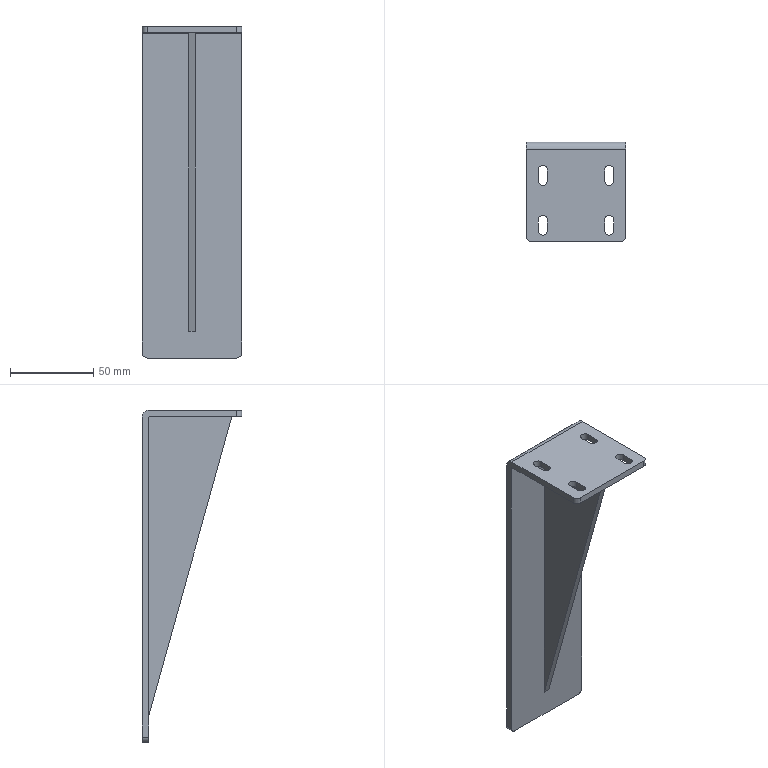Part | STEP file | HJDX-302 | 2 solids | 35 faces | box 60 x 60 x 200 mm | volume 78199 mm3 | plane 21 | cylinder 14 | commonest cylinder face diameters 5.5 x8 6 x4 1 x1 9 x1
STEP:
#1=CARTESIAN_POINT('',(-27.,56.,-200.));
#2=VERTEX_POINT('',#1);
#3=CARTESIAN_POINT('',(-30.,56.,-197.));
#4=VERTEX_POINT('',#3);
#5=CARTESIAN_POINT('',(-27.,56.,-197.));
#6=DIRECTION('',(0.,1.,0.));
#7=DIRECTION('',(0.,0.,1.));
#8=AXIS2_PLACEMENT_3D('',#5,#6,#7);
#9=CIRCLE('',#8,3.);
#10=EDGE_CURVE('',#2,#4,#9,.T.);
#11=ORIENTED_EDGE('',*,*,#10,.F.);
#12=CARTESIAN_POINT('',(27.,56.,-200.));
#13=VERTEX_POINT('',#12);
#14=CARTESIAN_POINT('',(30.,56.,-200.));
#15=DIRECTION('',(-1.,0.,0.));
#16=VECTOR('',#15,1000.);
#17=LINE('',#14,#16);
#18=EDGE_CURVE('',#13,#2,#17,.T.);
#19=ORIENTED_EDGE('',*,*,#18,.F.);
#20=CARTESIAN_POINT('',(30.,56.,-197.));
#21=VERTEX_POINT('',#20);
#22=CARTESIAN_POINT('',(27.,56.,-197.));
#23=DIRECTION('',(0.,1.,0.));
#24=DIRECTION('',(0.,0.,-1.));
#25=AXIS2_PLACEMENT_3D('',#22,#23,#24);
#26=CIRCLE('',#25,3.);
#27=EDGE_CURVE('',#21,#13,#26,.T.);
#28=ORIENTED_EDGE('',*,*,#27,.F.);
#29=CARTESIAN_POINT('',(30.,56.,-4.5));
#30=VERTEX_POINT('',#29);
#31=CARTESIAN_POINT('',(30.,56.,0.));
#32=DIRECTION('',(0.,0.,-1.));
#33=VECTOR('',#32,1000.);
#34=LINE('',#31,#33);
#35=EDGE_CURVE('',#30,#21,#34,.T.);
#36=ORIENTED_EDGE('',*,*,#35,.F.);
#37=CARTESIAN_POINT('',(-30.,56.,-4.5));
#38=VERTEX_POINT('',#37);
#39=CARTESIAN_POINT('',(30.,56.,-4.5));
#40=DIRECTION('',(1.,0.,0.));
#41=VECTOR('',#40,1000.);
#42=LINE('',#39,#41);
#43=EDGE_CURVE('',#38,#30,#42,.T.);
#44=ORIENTED_EDGE('',*,*,#43,.F.);
#45=CARTESIAN_POINT('',(-30.,56.,0.));
#46=DIRECTION('',(0.,0.,1.));
#47=VECTOR('',#46,1000.);
#48=LINE('',#45,#47);
#49=EDGE_CURVE('',#4,#38,#48,.T.);
#50=ORIENTED_EDGE('',*,*,#49,.F.);
#51=EDGE_LOOP('',(#11,#19,#28,#36,#44,#50));
#52=FACE_OUTER_BOUND('',#51,.T.);
#53=CARTESIAN_POINT('',(30.,56.,0.));
#54=DIRECTION('',(0.,1.,0.));
#55=DIRECTION('',(0.,0.,1.));
#56=AXIS2_PLACEMENT_3D('',#53,#54,#55);
#57=PLANE('',#56);
#58=ADVANCED_FACE('',(#52),#57,.F.);
#59=CARTESIAN_POINT('',(-30.,60.,-197.));
#60=VERTEX_POINT('',#59);
#61=CARTESIAN_POINT('',(-30.,55.5,-197.));
#62=DIRECTION('',(0.,1.,0.));
#63=VECTOR('',#62,1000.);
#64=LINE('',#61,#63);
#65=EDGE_CURVE('',#4,#60,#64,.T.);
#66=ORIENTED_EDGE('',*,*,#65,.F.);
#67=ORIENTED_EDGE('',*,*,#49,.T.);
#68=CARTESIAN_POINT('',(-30.,55.5,-4.));
#69=VERTEX_POINT('',#68);
#70=CARTESIAN_POINT('',(-30.,55.5,-4.5));
#71=DIRECTION('',(1.,0.,0.));
#72=DIRECTION('',(0.,0.,1.));
#73=AXIS2_PLACEMENT_3D('',#70,#71,#72);
#74=CIRCLE('',#73,0.5);
#75=EDGE_CURVE('',#38,#69,#74,.T.);
#76=ORIENTED_EDGE('',*,*,#75,.T.);
#77=CARTESIAN_POINT('',(-30.,3.,-4.));
#78=VERTEX_POINT('',#77);
#79=CARTESIAN_POINT('',(-30.,0.,-4.));
#80=DIRECTION('',(0.,-1.,0.));
#81=VECTOR('',#80,1000.);
#82=LINE('',#79,#81);
#83=EDGE_CURVE('',#69,#78,#82,.T.);
#84=ORIENTED_EDGE('',*,*,#83,.T.);
#85=CARTESIAN_POINT('',(-30.,3.,0.));
#86=VERTEX_POINT('',#85);
#87=CARTESIAN_POINT('',(-30.,3.,-4.5));
#88=DIRECTION('',(0.,0.,1.));
#89=VECTOR('',#88,1000.);
#90=LINE('',#87,#89);
#91=EDGE_CURVE('',#78,#86,#90,.T.);
#92=ORIENTED_EDGE('',*,*,#91,.T.);
#93=CARTESIAN_POINT('',(-30.,55.5,0.));
#94=VERTEX_POINT('',#93);
#95=CARTESIAN_POINT('',(-30.,56.,0.));
#96=DIRECTION('',(0.,1.,0.));
#97=VECTOR('',#96,1000.);
#98=LINE('',#95,#97);
#99=EDGE_CURVE('',#86,#94,#98,.T.);
#100=ORIENTED_EDGE('',*,*,#99,.T.);
#101=CARTESIAN_POINT('',(-30.,60.,-4.5));
#102=VERTEX_POINT('',#101);
#103=CARTESIAN_POINT('',(-30.,55.5,-4.5));
#104=DIRECTION('',(-1.,0.,0.));
#105=DIRECTION('',(0.,0.,1.));
#106=AXIS2_PLACEMENT_3D('',#103,#104,#105);
#107=CIRCLE('',#106,4.5);
#108=EDGE_CURVE('',#94,#102,#107,.T.);
#109=ORIENTED_EDGE('',*,*,#108,.T.);
#110=CARTESIAN_POINT('',(-30.,60.,-4.5));
#111=DIRECTION('',(0.,0.,1.));
#112=VECTOR('',#111,1000.);
#113=LINE('',#110,#112);
#114=EDGE_CURVE('',#60,#102,#113,.T.);
#115=ORIENTED_EDGE('',*,*,#114,.F.);
#116=EDGE_LOOP('',(#66,#67,#76,#84,#92,#100,#109,#115));
#117=FACE_OUTER_BOUND('',#116,.T.);
#118=CARTESIAN_POINT('',(-30.,55.5,-4.5));
#119=DIRECTION('',(1.,0.,0.));
#120=DIRECTION('',(0.,0.,-1.));
#121=AXIS2_PLACEMENT_3D('',#118,#119,#120);
#122=PLANE('',#121);
#123=ADVANCED_FACE('',(#117),#122,.F.);
#124=ORIENTED_EDGE('',*,*,#10,.T.);
#125=ORIENTED_EDGE('',*,*,#65,.T.);
#126=CARTESIAN_POINT('',(-27.,60.,-200.));
#127=VERTEX_POINT('',#126);
#128=CARTESIAN_POINT('',(-27.,60.,-197.));
#129=DIRECTION('',(0.,-1.,0.));
#130=DIRECTION('',(0.,0.,1.));
#131=AXIS2_PLACEMENT_3D('',#128,#129,#130);
#132=CIRCLE('',#131,3.);
#133=EDGE_CURVE('',#60,#127,#132,.T.);
#134=ORIENTED_EDGE('',*,*,#133,.T.);
#135=CARTESIAN_POINT('',(-27.,55.5,-200.));
#136=DIRECTION('',(0.,-1.,0.));
#137=VECTOR('',#136,1000.);
#138=LINE('',#135,#137);
#139=EDGE_CURVE('',#127,#2,#138,.T.);
#140=ORIENTED_EDGE('',*,*,#139,.T.);
#141=EDGE_LOOP('',(#124,#125,#134,#140));
#142=FACE_OUTER_BOUND('',#141,.T.);
#143=CARTESIAN_POINT('',(-27.,55.5,-197.));
#144=DIRECTION('',(0.,1.,0.));
#145=DIRECTION('',(0.,0.,1.));
#146=AXIS2_PLACEMENT_3D('',#143,#144,#145);
#147=CYLINDRICAL_SURFACE('',#146,3.);
#148=ADVANCED_FACE('',(#142),#147,.T.);
#149=CARTESIAN_POINT('',(27.,60.,-200.));
#150=VERTEX_POINT('',#149);
#151=CARTESIAN_POINT('',(30.,60.,-200.));
#152=DIRECTION('',(1.,0.,0.));
#153=VECTOR('',#152,1000.);
#154=LINE('',#151,#153);
#155=EDGE_CURVE('',#127,#150,#154,.T.);
#156=ORIENTED_EDGE('',*,*,#155,.T.);
#157=CARTESIAN_POINT('',(27.,60.,-200.));
#158=DIRECTION('',(0.,-1.,0.));
#159=VECTOR('',#158,1000.);
#160=LINE('',#157,#159);
#161=EDGE_CURVE('',#150,#13,#160,.T.);
#162=ORIENTED_EDGE('',*,*,#161,.T.);
#163=ORIENTED_EDGE('',*,*,#18,.T.);
#164=ORIENTED_EDGE('',*,*,#139,.F.);
#165=EDGE_LOOP('',(#156,#162,#163,#164));
#166=FACE_OUTER_BOUND('',#165,.T.);
#167=CARTESIAN_POINT('',(30.,60.,-200.));
#168=DIRECTION('',(0.,0.,-1.));
#169=DIRECTION('',(-1.,0.,0.));
#170=AXIS2_PLACEMENT_3D('',#167,#168,#169);
#171=PLANE('',#170);
#172=ADVANCED_FACE('',(#166),#171,.T.);
#173=ORIENTED_EDGE('',*,*,#27,.T.);
#174=ORIENTED_EDGE('',*,*,#161,.F.);
#175=CARTESIAN_POINT('',(30.,60.,-197.));
#176=VERTEX_POINT('',#175);
#177=CARTESIAN_POINT('',(27.,60.,-197.));
#178=DIRECTION('',(0.,-1.,0.));
#179=DIRECTION('',(0.,0.,-1.));
#180=AXIS2_PLACEMENT_3D('',#177,#178,#179);
#181=CIRCLE('',#180,3.);
#182=EDGE_CURVE('',#150,#176,#181,.T.);
#183=ORIENTED_EDGE('',*,*,#182,.T.);
#184=CARTESIAN_POINT('',(30.,60.,-197.));
#185=DIRECTION('',(0.,-1.,0.));
#186=VECTOR('',#185,1000.);
#187=LINE('',#184,#186);
#188=EDGE_CURVE('',#176,#21,#187,.T.);
#189=ORIENTED_EDGE('',*,*,#188,.T.);
#190=EDGE_LOOP('',(#173,#174,#183,#189));
#191=FACE_OUTER_BOUND('',#190,.T.);
#192=CARTESIAN_POINT('',(27.,60.,-197.));
#193=DIRECTION('',(0.,-1.,0.));
#194=DIRECTION('',(0.,0.,-1.));
#195=AXIS2_PLACEMENT_3D('',#192,#193,#194);
#196=CYLINDRICAL_SURFACE('',#195,3.);
#197=ADVANCED_FACE('',(#191),#196,.T.);
#198=CARTESIAN_POINT('',(30.,60.,-4.5));
#199=VERTEX_POINT('',#198);
#200=CARTESIAN_POINT('',(30.,60.,-4.));
#201=DIRECTION('',(0.,0.,1.));
#202=VECTOR('',#201,1000.);
#203=LINE('',#200,#202);
#204=EDGE_CURVE('',#176,#199,#203,.T.);
#205=ORIENTED_EDGE('',*,*,#204,.T.);
#206=CARTESIAN_POINT('',(30.,55.5,0.));
#207=VERTEX_POINT('',#206);
#208=CARTESIAN_POINT('',(30.,55.5,-4.5));
#209=DIRECTION('',(1.,0.,0.));
#210=DIRECTION('',(0.,0.,1.));
#211=AXIS2_PLACEMENT_3D('',#208,#209,#210);
#212=CIRCLE('',#211,4.5);
#213=EDGE_CURVE('',#199,#207,#212,.T.);
#214=ORIENTED_EDGE('',*,*,#213,.T.);
#215=CARTESIAN_POINT('',(30.,3.,0.));
#216=VERTEX_POINT('',#215);
#217=CARTESIAN_POINT('',(30.,55.5,0.));
#218=DIRECTION('',(0.,-1.,0.));
#219=VECTOR('',#218,1000.);
#220=LINE('',#217,#219);
#221=EDGE_CURVE('',#207,#216,#220,.T.);
#222=ORIENTED_EDGE('',*,*,#221,.T.);
#223=CARTESIAN_POINT('',(30.,3.,-4.));
#224=VERTEX_POINT('',#223);
#225=CARTESIAN_POINT('',(30.,3.,-4.5));
#226=DIRECTION('',(0.,0.,-1.));
#227=VECTOR('',#226,1000.);
#228=LINE('',#225,#227);
#229=EDGE_CURVE('',#216,#224,#228,.T.);
#230=ORIENTED_EDGE('',*,*,#229,.T.);
#231=CARTESIAN_POINT('',(30.,55.5,-4.));
#232=VERTEX_POINT('',#231);
#233=CARTESIAN_POINT('',(30.,0.,-4.));
#234=DIRECTION('',(0.,1.,0.));
#235=VECTOR('',#234,1000.);
#236=LINE('',#233,#235);
#237=EDGE_CURVE('',#224,#232,#236,.T.);
#238=ORIENTED_EDGE('',*,*,#237,.T.);
#239=CARTESIAN_POINT('',(30.,55.5,-4.5));
#240=DIRECTION('',(-1.,0.,0.));
#241=DIRECTION('',(0.,0.,1.));
#242=AXIS2_PLACEMENT_3D('',#239,#240,#241);
#243=CIRCLE('',#242,0.5);
#244=EDGE_CURVE('',#232,#30,#243,.T.);
#245=ORIENTED_EDGE('',*,*,#244,.T.);
#246=ORIENTED_EDGE('',*,*,#35,.T.);
#247=ORIENTED_EDGE('',*,*,#188,.F.);
#248=EDGE_LOOP('',(#205,#214,#222,#230,#238,#245,#246,#247));
#249=FACE_OUTER_BOUND('',#248,.T.);
#250=CARTESIAN_POINT('',(30.,55.5,-4.));
#251=DIRECTION('',(1.,0.,0.));
#252=DIRECTION('',(0.,0.,-1.));
#253=AXIS2_PLACEMENT_3D('',#250,#251,#252);
#254=PLANE('',#253);
#255=ADVANCED_FACE('',(#249),#254,.T.);
#256=ORIENTED_EDGE('',*,*,#43,.T.);
#257=ORIENTED_EDGE('',*,*,#244,.F.);
#258=CARTESIAN_POINT('',(30.,55.5,-4.));
#259=DIRECTION('',(1.,0.,0.));
#260=VECTOR('',#259,1000.);
#261=LINE('',#258,#260);
#262=EDGE_CURVE('',#69,#232,#261,.T.);
#263=ORIENTED_EDGE('',*,*,#262,.F.);
#264=ORIENTED_EDGE('',*,*,#75,.F.);
#265=EDGE_LOOP('',(#256,#257,#263,#264));
#266=FACE_OUTER_BOUND('',#265,.T.);
#267=CARTESIAN_POINT('',(30.,55.5,-4.5));
#268=DIRECTION('',(-1.,0.,0.));
#269=DIRECTION('',(0.,0.,1.));
#270=AXIS2_PLACEMENT_3D('',#267,#268,#269);
#271=CYLINDRICAL_SURFACE('',#270,0.5);
#272=ADVANCED_FACE('',(#266),#271,.F.);
#273=ORIENTED_EDGE('',*,*,#204,.F.);
#274=ORIENTED_EDGE('',*,*,#182,.F.);
#275=ORIENTED_EDGE('',*,*,#155,.F.);
#276=ORIENTED_EDGE('',*,*,#133,.F.);
#277=ORIENTED_EDGE('',*,*,#114,.T.);
#278=CARTESIAN_POINT('',(30.,60.,-4.5));
#279=DIRECTION('',(1.,0.,0.));
#280=VECTOR('',#279,1000.);
#281=LINE('',#278,#280);
#282=EDGE_CURVE('',#102,#199,#281,.T.);
#283=ORIENTED_EDGE('',*,*,#282,.T.);
#284=EDGE_LOOP('',(#273,#274,#275,#276,#277,#283));
#285=FACE_OUTER_BOUND('',#284,.T.);
#286=CARTESIAN_POINT('',(30.,60.,0.));
#287=DIRECTION('',(0.,1.,0.));
#288=DIRECTION('',(0.,0.,1.));
#289=AXIS2_PLACEMENT_3D('',#286,#287,#288);
#290=PLANE('',#289);
#291=ADVANCED_FACE('',(#285),#290,.T.);
#292=CARTESIAN_POINT('',(-22.75,6.75,-4.));
#293=VERTEX_POINT('',#292);
#294=CARTESIAN_POINT('',(-22.75,13.25,-4.));
#295=VERTEX_POINT('',#294);
#296=CARTESIAN_POINT('',(-22.75,0.,-4.));
#297=DIRECTION('',(0.,1.,0.));
#298=VECTOR('',#297,1000.);
#299=LINE('',#296,#298);
#300=EDGE_CURVE('',#293,#295,#299,.T.);
#301=ORIENTED_EDGE('',*,*,#300,.F.);
#302=CARTESIAN_POINT('',(-17.25,6.75,-4.));
#303=VERTEX_POINT('',#302);
#304=CARTESIAN_POINT('',(-20.,6.75,-4.));
#305=DIRECTION('',(0.,0.,-1.));
#306=DIRECTION('',(-1.,0.,0.));
#307=AXIS2_PLACEMENT_3D('',#304,#305,#306);
#308=CIRCLE('',#307,2.75);
#309=EDGE_CURVE('',#303,#293,#308,.T.);
#310=ORIENTED_EDGE('',*,*,#309,.F.);
#311=CARTESIAN_POINT('',(-17.25,13.25,-4.));
#312=VERTEX_POINT('',#311);
#313=CARTESIAN_POINT('',(-17.25,0.,-4.));
#314=DIRECTION('',(0.,-1.,0.));
#315=VECTOR('',#314,1000.);
#316=LINE('',#313,#315);
#317=EDGE_CURVE('',#312,#303,#316,.T.);
#318=ORIENTED_EDGE('',*,*,#317,.F.);
#319=CARTESIAN_POINT('',(-20.,13.25,-4.));
#320=DIRECTION('',(0.,0.,-1.));
#321=DIRECTION('',(-1.,0.,0.));
#322=AXIS2_PLACEMENT_3D('',#319,#320,#321);
#323=CIRCLE('',#322,2.75);
#324=EDGE_CURVE('',#295,#312,#323,.T.);
#325=ORIENTED_EDGE('',*,*,#324,.F.);
#326=EDGE_LOOP('',(#301,#310,#318,#325));
#327=FACE_BOUND('',#326,.T.);
#328=CARTESIAN_POINT('',(-22.75,36.75,-4.));
#329=VERTEX_POINT('',#328);
#330=CARTESIAN_POINT('',(-22.75,43.25,-4.));
#331=VERTEX_POINT('',#330);
#332=CARTESIAN_POINT('',(-22.75,0.,-4.));
#333=DIRECTION('',(0.,1.,0.));
#334=VECTOR('',#333,1000.);
#335=LINE('',#332,#334);
#336=EDGE_CURVE('',#329,#331,#335,.T.);
#337=ORIENTED_EDGE('',*,*,#336,.F.);
#338=CARTESIAN_POINT('',(-17.25,36.75,-4.));
#339=VERTEX_POINT('',#338);
#340=CARTESIAN_POINT('',(-20.,36.75,-4.));
#341=DIRECTION('',(0.,0.,-1.));
#342=DIRECTION('',(-1.,0.,0.));
#343=AXIS2_PLACEMENT_3D('',#340,#341,#342);
#344=CIRCLE('',#343,2.75);
#345=EDGE_CURVE('',#339,#329,#344,.T.);
#346=ORIENTED_EDGE('',*,*,#345,.F.);
#347=CARTESIAN_POINT('',(-17.25,43.25,-4.));
#348=VERTEX_POINT('',#347);
#349=CARTESIAN_POINT('',(-17.25,0.,-4.));
#350=DIRECTION('',(0.,-1.,0.));
#351=VECTOR('',#350,1000.);
#352=LINE('',#349,#351);
#353=EDGE_CURVE('',#348,#339,#352,.T.);
#354=ORIENTED_EDGE('',*,*,#353,.F.);
#355=CARTESIAN_POINT('',(-20.,43.25,-4.));
#356=DIRECTION('',(0.,0.,-1.));
#357=DIRECTION('',(-1.,0.,0.));
#358=AXIS2_PLACEMENT_3D('',#355,#356,#357);
#359=CIRCLE('',#358,2.75);
#360=EDGE_CURVE('',#331,#348,#359,.T.);
#361=ORIENTED_EDGE('',*,*,#360,.F.);
#362=EDGE_LOOP('',(#337,#346,#354,#361));
#363=FACE_BOUND('',#362,.T.);
#364=CARTESIAN_POINT('',(27.,0.,-4.));
#365=VERTEX_POINT('',#364);
#366=CARTESIAN_POINT('',(27.,3.,-4.));
#367=DIRECTION('',(0.,0.,1.));
#368=DIRECTION('',(1.,0.,0.));
#369=AXIS2_PLACEMENT_3D('',#366,#367,#368);
#370=CIRCLE('',#369,3.);
#371=EDGE_CURVE('',#365,#224,#370,.T.);
#372=ORIENTED_EDGE('',*,*,#371,.F.);
#373=CARTESIAN_POINT('',(-27.,0.,-4.));
#374=VERTEX_POINT('',#373);
#375=CARTESIAN_POINT('',(30.,0.,-4.));
#376=DIRECTION('',(1.,0.,0.));
#377=VECTOR('',#376,1000.);
#378=LINE('',#375,#377);
#379=EDGE_CURVE('',#374,#365,#378,.T.);
#380=ORIENTED_EDGE('',*,*,#379,.F.);
#381=CARTESIAN_POINT('',(-27.,3.,-4.));
#382=DIRECTION('',(0.,0.,1.));
#383=DIRECTION('',(1.,0.,0.));
#384=AXIS2_PLACEMENT_3D('',#381,#382,#383);
#385=CIRCLE('',#384,3.);
#386=EDGE_CURVE('',#78,#374,#385,.T.);
#387=ORIENTED_EDGE('',*,*,#386,.F.);
#388=ORIENTED_EDGE('',*,*,#83,.F.);
#389=ORIENTED_EDGE('',*,*,#262,.T.);
#390=ORIENTED_EDGE('',*,*,#237,.F.);
#391=EDGE_LOOP('',(#372,#380,#387,#388,#389,#390));
#392=FACE_OUTER_BOUND('',#391,.T.);
#393=CARTESIAN_POINT('',(17.25,36.75,-4.));
#394=VERTEX_POINT('',#393);
#395=CARTESIAN_POINT('',(17.25,43.25,-4.));
#396=VERTEX_POINT('',#395);
#397=CARTESIAN_POINT('',(17.25,0.,-4.));
#398=DIRECTION('',(0.,1.,0.));
#399=VECTOR('',#398,1000.);
#400=LINE('',#397,#399);
#401=EDGE_CURVE('',#394,#396,#400,.T.);
#402=ORIENTED_EDGE('',*,*,#401,.F.);
#403=CARTESIAN_POINT('',(22.75,36.75,-4.));
#404=VERTEX_POINT('',#403);
#405=CARTESIAN_POINT('',(20.,36.75,-4.));
#406=DIRECTION('',(0.,0.,-1.));
#407=DIRECTION('',(-1.,0.,0.));
#408=AXIS2_PLACEMENT_3D('',#405,#406,#407);
#409=CIRCLE('',#408,2.75);
#410=EDGE_CURVE('',#404,#394,#409,.T.);
#411=ORIENTED_EDGE('',*,*,#410,.F.);
#412=CARTESIAN_POINT('',(22.75,43.25,-4.));
#413=VERTEX_POINT('',#412);
#414=CARTESIAN_POINT('',(22.75,0.,-4.));
#415=DIRECTION('',(0.,-1.,0.));
#416=VECTOR('',#415,1000.);
#417=LINE('',#414,#416);
#418=EDGE_CURVE('',#413,#404,#417,.T.);
#419=ORIENTED_EDGE('',*,*,#418,.F.);
#420=CARTESIAN_POINT('',(20.,43.25,-4.));
#421=DIRECTION('',(0.,0.,-1.));
#422=DIRECTION('',(-1.,0.,0.));
#423=AXIS2_PLACEMENT_3D('',#420,#421,#422);
#424=CIRCLE('',#423,2.75);
#425=EDGE_CURVE('',#396,#413,#424,.T.);
#426=ORIENTED_EDGE('',*,*,#425,.F.);
#427=EDGE_LOOP('',(#402,#411,#419,#426));
#428=FACE_BOUND('',#427,.T.);
#429=CARTESIAN_POINT('',(22.75,13.25,-4.));
#430=VERTEX_POINT('',#429);
#431=CARTESIAN_POINT('',(22.75,6.75,-4.));
#432=VERTEX_POINT('',#431);
#433=CARTESIAN_POINT('',(22.75,0.,-4.));
#434=DIRECTION('',(0.,-1.,0.));
#435=VECTOR('',#434,1000.);
#436=LINE('',#433,#435);
#437=EDGE_CURVE('',#430,#432,#436,.T.);
#438=ORIENTED_EDGE('',*,*,#437,.F.);
#439=CARTESIAN_POINT('',(17.25,13.25,-4.));
#440=VERTEX_POINT('',#439);
#441=CARTESIAN_POINT('',(20.,13.25,-4.));
#442=DIRECTION('',(0.,0.,-1.));
#443=DIRECTION('',(-1.,0.,0.));
#444=AXIS2_PLACEMENT_3D('',#441,#442,#443);
#445=CIRCLE('',#444,2.75);
#446=EDGE_CURVE('',#440,#430,#445,.T.);
#447=ORIENTED_EDGE('',*,*,#446,.F.);
#448=CARTESIAN_POINT('',(17.25,6.75,-4.));
#449=VERTEX_POINT('',#448);
#450=CARTESIAN_POINT('',(17.25,0.,-4.));
#451=DIRECTION('',(0.,1.,0.));
#452=VECTOR('',#451,1000.);
#453=LINE('',#450,#452);
#454=EDGE_CURVE('',#449,#440,#453,.T.);
#455=ORIENTED_EDGE('',*,*,#454,.F.);
#456=CARTESIAN_POINT('',(20.,6.75,-4.));
#457=DIRECTION('',(0.,0.,-1.));
#458=DIRECTION('',(-1.,0.,0.));
#459=AXIS2_PLACEMENT_3D('',#456,#457,#458);
#460=CIRCLE('',#459,2.75);
#461=EDGE_CURVE('',#432,#449,#460,.T.);
#462=ORIENTED_EDGE('',*,*,#461,.F.);
#463=EDGE_LOOP('',(#438,#447,#455,#462));
#464=FACE_BOUND('',#463,.T.);
#465=CARTESIAN_POINT('',(30.,0.,-4.));
#466=DIRECTION('',(0.,0.,1.));
#467=DIRECTION('',(1.,0.,0.));
#468=AXIS2_PLACEMENT_3D('',#465,#466,#467);
#469=PLANE('',#468);
#470=ADVANCED_FACE('',(#327,#363,#392,#428,#464),#469,.F.);
#471=ORIENTED_EDGE('',*,*,#213,.F.);
#472=ORIENTED_EDGE('',*,*,#282,.F.);
#473=ORIENTED_EDGE('',*,*,#108,.F.);
#474=CARTESIAN_POINT('',(30.,55.5,0.));
#475=DIRECTION('',(1.,0.,0.));
#476=VECTOR('',#475,1000.);
#477=LINE('',#474,#476);
#478=EDGE_CURVE('',#94,#207,#477,.T.);
#479=ORIENTED_EDGE('',*,*,#478,.T.);
#480=EDGE_LOOP('',(#471,#472,#473,#479));
#481=FACE_OUTER_BOUND('',#480,.T.);
#482=CARTESIAN_POINT('',(30.,55.5,-4.5));
#483=DIRECTION('',(-1.,0.,0.));
#484=DIRECTION('',(0.,0.,1.));
#485=AXIS2_PLACEMENT_3D('',#482,#483,#484);
#486=CYLINDRICAL_SURFACE('',#485,4.5);
#487=ADVANCED_FACE('',(#481),#486,.T.);
#488=CARTESIAN_POINT('',(-17.25,13.25,0.));
#489=VERTEX_POINT('',#488);
#490=CARTESIAN_POINT('',(-17.25,13.25,-4.));
#491=DIRECTION('',(0.,0.,-1.));
#492=VECTOR('',#491,1000.);
#493=LINE('',#490,#492);
#494=EDGE_CURVE('',#489,#312,#493,.T.);
#495=ORIENTED_EDGE('',*,*,#494,.F.);
#496=CARTESIAN_POINT('',(-22.75,13.25,0.));
#497=VERTEX_POINT('',#496);
#498=CARTESIAN_POINT('',(-20.,13.25,0.));
#499=DIRECTION('',(0.,0.,-1.));
#500=DIRECTION('',(-1.,0.,0.));
#501=AXIS2_PLACEMENT_3D('',#498,#499,#500);
#502=CIRCLE('',#501,2.75);
#503=EDGE_CURVE('',#497,#489,#502,.T.);
#504=ORIENTED_EDGE('',*,*,#503,.F.);
#505=CARTESIAN_POINT('',(-22.75,13.25,-4.));
#506=DIRECTION('',(0.,0.,1.));
#507=VECTOR('',#506,1000.);
#508=LINE('',#505,#507);
#509=EDGE_CURVE('',#295,#497,#508,.T.);
#510=ORIENTED_EDGE('',*,*,#509,.F.);
#511=ORIENTED_EDGE('',*,*,#324,.T.);
#512=EDGE_LOOP('',(#495,#504,#510,#511));
#513=FACE_OUTER_BOUND('',#512,.T.);
#514=CARTESIAN_POINT('',(-20.,13.25,-4.));
#515=DIRECTION('',(0.,0.,-1.));
#516=DIRECTION('',(-1.,0.,0.));
#517=AXIS2_PLACEMENT_3D('',#514,#515,#516);
#518=CYLINDRICAL_SURFACE('',#517,2.75);
#519=ADVANCED_FACE('',(#513),#518,.F.);
#520=CARTESIAN_POINT('',(-22.75,6.75,0.));
#521=VERTEX_POINT('',#520);
#522=CARTESIAN_POINT('',(-22.75,6.75,0.));
#523=DIRECTION('',(0.,1.,0.));
#524=VECTOR('',#523,1000.);
#525=LINE('',#522,#524);
#526=EDGE_CURVE('',#521,#497,#525,.T.);
#527=ORIENTED_EDGE('',*,*,#526,.F.);
#528=CARTESIAN_POINT('',(-22.75,6.75,-4.));
#529=DIRECTION('',(0.,0.,1.));
#530=VECTOR('',#529,1000.);
#531=LINE('',#528,#530);
#532=EDGE_CURVE('',#293,#521,#531,.T.);
#533=ORIENTED_EDGE('',*,*,#532,.F.);
#534=ORIENTED_EDGE('',*,*,#300,.T.);
#535=ORIENTED_EDGE('',*,*,#509,.T.);
#536=EDGE_LOOP('',(#527,#533,#534,#535));
#537=FACE_OUTER_BOUND('',#536,.T.);
#538=CARTESIAN_POINT('',(-22.75,6.75,-4.));
#539=DIRECTION('',(-1.,0.,0.));
#540=DIRECTION('',(0.,0.,1.));
#541=AXIS2_PLACEMENT_3D('',#538,#539,#540);
#542=PLANE('',#541);
#543=ADVANCED_FACE('',(#537),#542,.F.);
#544=CARTESIAN_POINT('',(-17.25,6.75,0.));
#545=VERTEX_POINT('',#544);
#546=CARTESIAN_POINT('',(-17.25,6.75,-4.));
#547=DIRECTION('',(0.,0.,1.));
#548=VECTOR('',#547,1000.);
#549=LINE('',#546,#548);
#550=EDGE_CURVE('',#303,#545,#549,.T.);
#551=ORIENTED_EDGE('',*,*,#550,.F.);
#552=ORIENTED_EDGE('',*,*,#309,.T.);
#553=ORIENTED_EDGE('',*,*,#532,.T.);
#554=CARTESIAN_POINT('',(-20.,6.75,0.));
#555=DIRECTION('',(0.,0.,-1.));
#556=DIRECTION('',(-1.,0.,0.));
#557=AXIS2_PLACEMENT_3D('',#554,#555,#556);
#558=CIRCLE('',#557,2.75);
#559=EDGE_CURVE('',#545,#521,#558,.T.);
#560=ORIENTED_EDGE('',*,*,#559,.F.);
#561=EDGE_LOOP('',(#551,#552,#553,#560));
#562=FACE_OUTER_BOUND('',#561,.T.);
#563=CARTESIAN_POINT('',(-20.,6.75,-4.));
#564=DIRECTION('',(0.,0.,-1.));
#565=DIRECTION('',(-1.,0.,0.));
#566=AXIS2_PLACEMENT_3D('',#563,#564,#565);
#567=CYLINDRICAL_SURFACE('',#566,2.75);
#568=ADVANCED_FACE('',(#562),#567,.F.);
#569=ORIENTED_EDGE('',*,*,#550,.T.);
#570=CARTESIAN_POINT('',(-17.25,6.75,0.));
#571=DIRECTION('',(0.,1.,0.));
#572=VECTOR('',#571,1000.);
#573=LINE('',#570,#572);
#574=EDGE_CURVE('',#545,#489,#573,.T.);
#575=ORIENTED_EDGE('',*,*,#574,.T.);
#576=ORIENTED_EDGE('',*,*,#494,.T.);
#577=ORIENTED_EDGE('',*,*,#317,.T.);
#578=EDGE_LOOP('',(#569,#575,#576,#577));
#579=FACE_OUTER_BOUND('',#578,.T.);
#580=CARTESIAN_POINT('',(-17.25,6.75,0.));
#581=DIRECTION('',(-1.,0.,0.));
#582=DIRECTION('',(0.,0.,1.));
#583=AXIS2_PLACEMENT_3D('',#580,#581,#582);
#584=PLANE('',#583);
#585=ADVANCED_FACE('',(#579),#584,.T.);
#586=CARTESIAN_POINT('',(-17.25,43.25,0.));
#587=VERTEX_POINT('',#586);
#588=CARTESIAN_POINT('',(-17.25,43.25,-4.));
#589=DIRECTION('',(0.,0.,-1.));
#590=VECTOR('',#589,1000.);
#591=LINE('',#588,#590);
#592=EDGE_CURVE('',#587,#348,#591,.T.);
#593=ORIENTED_EDGE('',*,*,#592,.F.);
#594=CARTESIAN_POINT('',(-22.75,43.25,0.));
#595=VERTEX_POINT('',#594);
#596=CARTESIAN_POINT('',(-20.,43.25,0.));
#597=DIRECTION('',(0.,0.,-1.));
#598=DIRECTION('',(-1.,0.,0.));
#599=AXIS2_PLACEMENT_3D('',#596,#597,#598);
#600=CIRCLE('',#599,2.75);
#601=EDGE_CURVE('',#595,#587,#600,.T.);
#602=ORIENTED_EDGE('',*,*,#601,.F.);
#603=CARTESIAN_POINT('',(-22.75,43.25,-4.));
#604=DIRECTION('',(0.,0.,1.));
#605=VECTOR('',#604,1000.);
#606=LINE('',#603,#605);
#607=EDGE_CURVE('',#331,#595,#606,.T.);
#608=ORIENTED_EDGE('',*,*,#607,.F.);
#609=ORIENTED_EDGE('',*,*,#360,.T.);
#610=EDGE_LOOP('',(#593,#602,#608,#609));
#611=FACE_OUTER_BOUND('',#610,.T.);
#612=CARTESIAN_POINT('',(-20.,43.25,-4.));
#613=DIRECTION('',(0.,0.,-1.));
#614=DIRECTION('',(-1.,0.,0.));
#615=AXIS2_PLACEMENT_3D('',#612,#613,#614);
#616=CYLINDRICAL_SURFACE('',#615,2.75);
#617=ADVANCED_FACE('',(#611),#616,.F.);
#618=CARTESIAN_POINT('',(-22.75,36.75,0.));
#619=VERTEX_POINT('',#618);
#620=CARTESIAN_POINT('',(-22.75,36.75,0.));
#621=DIRECTION('',(0.,1.,0.));
#622=VECTOR('',#621,1000.);
#623=LINE('',#620,#622);
#624=EDGE_CURVE('',#619,#595,#623,.T.);
#625=ORIENTED_EDGE('',*,*,#624,.F.);
#626=CARTESIAN_POINT('',(-22.75,36.75,-4.));
#627=DIRECTION('',(0.,0.,1.));
#628=VECTOR('',#627,1000.);
#629=LINE('',#626,#628);
#630=EDGE_CURVE('',#329,#619,#629,.T.);
#631=ORIENTED_EDGE('',*,*,#630,.F.);
#632=ORIENTED_EDGE('',*,*,#336,.T.);
#633=ORIENTED_EDGE('',*,*,#607,.T.);
#634=EDGE_LOOP('',(#625,#631,#632,#633));
#635=FACE_OUTER_BOUND('',#634,.T.);
#636=CARTESIAN_POINT('',(-22.75,36.75,-4.));
#637=DIRECTION('',(-1.,0.,0.));
#638=DIRECTION('',(0.,0.,1.));
#639=AXIS2_PLACEMENT_3D('',#636,#637,#638);
#640=PLANE('',#639);
#641=ADVANCED_FACE('',(#635),#640,.F.);
#642=CARTESIAN_POINT('',(-17.25,36.75,0.));
#643=VERTEX_POINT('',#642);
#644=CARTESIAN_POINT('',(-17.25,36.75,-4.));
#645=DIRECTION('',(0.,0.,1.));
#646=VECTOR('',#645,1000.);
#647=LINE('',#644,#646);
#648=EDGE_CURVE('',#339,#643,#647,.T.);
#649=ORIENTED_EDGE('',*,*,#648,.F.);
#650=ORIENTED_EDGE('',*,*,#345,.T.);
#651=ORIENTED_EDGE('',*,*,#630,.T.);
#652=CARTESIAN_POINT('',(-20.,36.75,0.));
#653=DIRECTION('',(0.,0.,-1.));
#654=DIRECTION('',(-1.,0.,0.));
#655=AXIS2_PLACEMENT_3D('',#652,#653,#654);
#656=CIRCLE('',#655,2.75);
#657=EDGE_CURVE('',#643,#619,#656,.T.);
#658=ORIENTED_EDGE('',*,*,#657,.F.);
#659=EDGE_LOOP('',(#649,#650,#651,#658));
#660=FACE_OUTER_BOUND('',#659,.T.);
#661=CARTESIAN_POINT('',(-20.,36.75,-4.));
#662=DIRECTION('',(0.,0.,-1.));
#663=DIRECTION('',(-1.,0.,0.));
#664=AXIS2_PLACEMENT_3D('',#661,#662,#663);
#665=CYLINDRICAL_SURFACE('',#664,2.75);
#666=ADVANCED_FACE('',(#660),#665,.F.);
#667=ORIENTED_EDGE('',*,*,#648,.T.);
#668=CARTESIAN_POINT('',(-17.25,36.75,0.));
#669=DIRECTION('',(0.,1.,0.));
#670=VECTOR('',#669,1000.);
#671=LINE('',#668,#670);
#672=EDGE_CURVE('',#643,#587,#671,.T.);
#673=ORIENTED_EDGE('',*,*,#672,.T.);
#674=ORIENTED_EDGE('',*,*,#592,.T.);
#675=ORIENTED_EDGE('',*,*,#353,.T.);
#676=EDGE_LOOP('',(#667,#673,#674,#675));
#677=FACE_OUTER_BOUND('',#676,.T.);
#678=CARTESIAN_POINT('',(-17.25,36.75,0.));
#679=DIRECTION('',(-1.,0.,0.));
#680=DIRECTION('',(0.,0.,1.));
#681=AXIS2_PLACEMENT_3D('',#678,#679,#680);
#682=PLANE('',#681);
#683=ADVANCED_FACE('',(#677),#682,.T.);
#684=CARTESIAN_POINT('',(27.,0.,0.));
#685=VERTEX_POINT('',#684);
#686=CARTESIAN_POINT('',(27.,3.,0.));
#687=DIRECTION('',(0.,0.,-1.));
#688=DIRECTION('',(1.,0.,0.));
#689=AXIS2_PLACEMENT_3D('',#686,#687,#688);
#690=CIRCLE('',#689,3.);
#691=EDGE_CURVE('',#216,#685,#690,.T.);
#692=ORIENTED_EDGE('',*,*,#691,.T.);
#693=CARTESIAN_POINT('',(27.,0.,-4.));
#694=DIRECTION('',(0.,0.,-1.));
#695=VECTOR('',#694,1000.);
#696=LINE('',#693,#695);
#697=EDGE_CURVE('',#685,#365,#696,.T.);
#698=ORIENTED_EDGE('',*,*,#697,.T.);
#699=ORIENTED_EDGE('',*,*,#371,.T.);
#700=ORIENTED_EDGE('',*,*,#229,.F.);
#701=EDGE_LOOP('',(#692,#698,#699,#700));
#702=FACE_OUTER_BOUND('',#701,.T.);
#703=CARTESIAN_POINT('',(27.,3.,-4.));
#704=DIRECTION('',(0.,0.,1.));
#705=DIRECTION('',(1.,0.,0.));
#706=AXIS2_PLACEMENT_3D('',#703,#704,#705);
#707=CYLINDRICAL_SURFACE('',#706,3.);
#708=ADVANCED_FACE('',(#702),#707,.T.);
#709=CARTESIAN_POINT('',(-27.,0.,0.));
#710=VERTEX_POINT('',#709);
#711=CARTESIAN_POINT('',(30.,0.,0.));
#712=DIRECTION('',(-1.,0.,0.));
#713=VECTOR('',#712,1000.);
#714=LINE('',#711,#713);
#715=EDGE_CURVE('',#685,#710,#714,.T.);
#716=ORIENTED_EDGE('',*,*,#715,.T.);
#717=CARTESIAN_POINT('',(-27.,0.,-4.));
#718=DIRECTION('',(0.,0.,-1.));
#719=VECTOR('',#718,1000.);
#720=LINE('',#717,#719);
#721=EDGE_CURVE('',#710,#374,#720,.T.);
#722=ORIENTED_EDGE('',*,*,#721,.T.);
#723=ORIENTED_EDGE('',*,*,#379,.T.);
#724=ORIENTED_EDGE('',*,*,#697,.F.);
#725=EDGE_LOOP('',(#716,#722,#723,#724));
#726=FACE_OUTER_BOUND('',#725,.T.);
#727=CARTESIAN_POINT('',(30.,0.,-4.));
#728=DIRECTION('',(0.,-1.,0.));
#729=DIRECTION('',(0.,0.,-1.));
#730=AXIS2_PLACEMENT_3D('',#727,#728,#729);
#731=PLANE('',#730);
#732=ADVANCED_FACE('',(#726),#731,.T.);
#733=CARTESIAN_POINT('',(-27.,3.,0.));
#734=DIRECTION('',(0.,0.,-1.));
#735=DIRECTION('',(1.,0.,0.));
#736=AXIS2_PLACEMENT_3D('',#733,#734,#735);
#737=CIRCLE('',#736,3.);
#738=EDGE_CURVE('',#710,#86,#737,.T.);
#739=ORIENTED_EDGE('',*,*,#738,.T.);
#740=ORIENTED_EDGE('',*,*,#91,.F.);
#741=ORIENTED_EDGE('',*,*,#386,.T.);
#742=ORIENTED_EDGE('',*,*,#721,.F.);
#743=EDGE_LOOP('',(#739,#740,#741,#742));
#744=FACE_OUTER_BOUND('',#743,.T.);
#745=CARTESIAN_POINT('',(-27.,3.,-4.5));
#746=DIRECTION('',(0.,0.,1.));
#747=DIRECTION('',(1.,0.,0.));
#748=AXIS2_PLACEMENT_3D('',#745,#746,#747);
#749=CYLINDRICAL_SURFACE('',#748,3.);
#750=ADVANCED_FACE('',(#744),#749,.T.);
#751=CARTESIAN_POINT('',(22.75,43.25,0.));
#752=VERTEX_POINT('',#751);
#753=CARTESIAN_POINT('',(22.75,43.25,-4.));
#754=DIRECTION('',(0.,0.,-1.));
#755=VECTOR('',#754,1000.);
#756=LINE('',#753,#755);
#757=EDGE_CURVE('',#752,#413,#756,.T.);
#758=ORIENTED_EDGE('',*,*,#757,.F.);
#759=CARTESIAN_POINT('',(17.25,43.25,0.));
#760=VERTEX_POINT('',#759);
#761=CARTESIAN_POINT('',(20.,43.25,0.));
#762=DIRECTION('',(0.,0.,-1.));
#763=DIRECTION('',(-1.,0.,0.));
#764=AXIS2_PLACEMENT_3D('',#761,#762,#763);
#765=CIRCLE('',#764,2.75);
#766=EDGE_CURVE('',#760,#752,#765,.T.);
#767=ORIENTED_EDGE('',*,*,#766,.F.);
#768=CARTESIAN_POINT('',(17.25,43.25,-4.));
#769=DIRECTION('',(0.,0.,1.));
#770=VECTOR('',#769,1000.);
#771=LINE('',#768,#770);
#772=EDGE_CURVE('',#396,#760,#771,.T.);
#773=ORIENTED_EDGE('',*,*,#772,.F.);
#774=ORIENTED_EDGE('',*,*,#425,.T.);
#775=EDGE_LOOP('',(#758,#767,#773,#774));
#776=FACE_OUTER_BOUND('',#775,.T.);
#777=CARTESIAN_POINT('',(20.,43.25,-4.));
#778=DIRECTION('',(0.,0.,-1.));
#779=DIRECTION('',(-1.,0.,0.));
#780=AXIS2_PLACEMENT_3D('',#777,#778,#779);
#781=CYLINDRICAL_SURFACE('',#780,2.75);
#782=ADVANCED_FACE('',(#776),#781,.F.);
#783=CARTESIAN_POINT('',(17.25,36.75,0.));
#784=VERTEX_POINT('',#783);
#785=CARTESIAN_POINT('',(17.25,36.75,0.));
#786=DIRECTION('',(0.,1.,0.));
#787=VECTOR('',#786,1000.);
#788=LINE('',#785,#787);
#789=EDGE_CURVE('',#784,#760,#788,.T.);
#790=ORIENTED_EDGE('',*,*,#789,.F.);
#791=CARTESIAN_POINT('',(17.25,36.75,-4.));
#792=DIRECTION('',(0.,0.,1.));
#793=VECTOR('',#792,1000.);
#794=LINE('',#791,#793);
#795=EDGE_CURVE('',#394,#784,#794,.T.);
#796=ORIENTED_EDGE('',*,*,#795,.F.);
#797=ORIENTED_EDGE('',*,*,#401,.T.);
#798=ORIENTED_EDGE('',*,*,#772,.T.);
#799=EDGE_LOOP('',(#790,#796,#797,#798));
#800=FACE_OUTER_BOUND('',#799,.T.);
#801=CARTESIAN_POINT('',(17.25,36.75,-4.));
#802=DIRECTION('',(-1.,0.,0.));
#803=DIRECTION('',(0.,0.,1.));
#804=AXIS2_PLACEMENT_3D('',#801,#802,#803);
#805=PLANE('',#804);
#806=ADVANCED_FACE('',(#800),#805,.F.);
#807=CARTESIAN_POINT('',(22.75,36.75,0.));
#808=VERTEX_POINT('',#807);
#809=CARTESIAN_POINT('',(22.75,36.75,-4.));
#810=DIRECTION('',(0.,0.,1.));
#811=VECTOR('',#810,1000.);
#812=LINE('',#809,#811);
#813=EDGE_CURVE('',#404,#808,#812,.T.);
#814=ORIENTED_EDGE('',*,*,#813,.F.);
#815=ORIENTED_EDGE('',*,*,#410,.T.);
#816=ORIENTED_EDGE('',*,*,#795,.T.);
#817=CARTESIAN_POINT('',(20.,36.75,0.));
#818=DIRECTION('',(0.,0.,-1.));
#819=DIRECTION('',(-1.,0.,0.));
#820=AXIS2_PLACEMENT_3D('',#817,#818,#819);
#821=CIRCLE('',#820,2.75);
#822=EDGE_CURVE('',#808,#784,#821,.T.);
#823=ORIENTED_EDGE('',*,*,#822,.F.);
#824=EDGE_LOOP('',(#814,#815,#816,#823));
#825=FACE_OUTER_BOUND('',#824,.T.);
#826=CARTESIAN_POINT('',(20.,36.75,-4.));
#827=DIRECTION('',(0.,0.,-1.));
#828=DIRECTION('',(-1.,0.,0.));
#829=AXIS2_PLACEMENT_3D('',#826,#827,#828);
#830=CYLINDRICAL_SURFACE('',#829,2.75);
#831=ADVANCED_FACE('',(#825),#830,.F.);
#832=ORIENTED_EDGE('',*,*,#813,.T.);
#833=CARTESIAN_POINT('',(22.75,36.75,0.));
#834=DIRECTION('',(0.,1.,0.));
#835=VECTOR('',#834,1000.);
#836=LINE('',#833,#835);
#837=EDGE_CURVE('',#808,#752,#836,.T.);
#838=ORIENTED_EDGE('',*,*,#837,.T.);
#839=ORIENTED_EDGE('',*,*,#757,.T.);
#840=ORIENTED_EDGE('',*,*,#418,.T.);
#841=EDGE_LOOP('',(#832,#838,#839,#840));
#842=FACE_OUTER_BOUND('',#841,.T.);
#843=CARTESIAN_POINT('',(22.75,36.75,0.));
#844=DIRECTION('',(-1.,0.,0.));
#845=DIRECTION('',(0.,0.,1.));
#846=AXIS2_PLACEMENT_3D('',#843,#844,#845);
#847=PLANE('',#846);
#848=ADVANCED_FACE('',(#842),#847,.T.);
#849=CARTESIAN_POINT('',(22.75,6.75,0.));
#850=VERTEX_POINT('',#849);
#851=CARTESIAN_POINT('',(22.75,6.75,-4.));
#852=DIRECTION('',(0.,0.,1.));
#853=VECTOR('',#852,1000.);
#854=LINE('',#851,#853);
#855=EDGE_CURVE('',#432,#850,#854,.T.);
#856=ORIENTED_EDGE('',*,*,#855,.F.);
#857=ORIENTED_EDGE('',*,*,#461,.T.);
#858=CARTESIAN_POINT('',(17.25,6.75,0.));
#859=VERTEX_POINT('',#858);
#860=CARTESIAN_POINT('',(17.25,6.75,-4.));
#861=DIRECTION('',(0.,0.,-1.));
#862=VECTOR('',#861,1000.);
#863=LINE('',#860,#862);
#864=EDGE_CURVE('',#859,#449,#863,.T.);
#865=ORIENTED_EDGE('',*,*,#864,.F.);
#866=CARTESIAN_POINT('',(20.,6.75,0.));
#867=DIRECTION('',(0.,0.,-1.));
#868=DIRECTION('',(-1.,0.,0.));
#869=AXIS2_PLACEMENT_3D('',#866,#867,#868);
#870=CIRCLE('',#869,2.75);
#871=EDGE_CURVE('',#850,#859,#870,.T.);
#872=ORIENTED_EDGE('',*,*,#871,.F.);
#873=EDGE_LOOP('',(#856,#857,#865,#872));
#874=FACE_OUTER_BOUND('',#873,.T.);
#875=CARTESIAN_POINT('',(20.,6.75,-4.));
#876=DIRECTION('',(0.,0.,-1.));
#877=DIRECTION('',(-1.,0.,0.));
#878=AXIS2_PLACEMENT_3D('',#875,#876,#877);
#879=CYLINDRICAL_SURFACE('',#878,2.75);
#880=ADVANCED_FACE('',(#874),#879,.F.);
#881=ORIENTED_EDGE('',*,*,#855,.T.);
#882=CARTESIAN_POINT('',(22.75,13.25,0.));
#883=VERTEX_POINT('',#882);
#884=CARTESIAN_POINT('',(22.75,6.75,0.));
#885=DIRECTION('',(0.,1.,0.));
#886=VECTOR('',#885,1000.);
#887=LINE('',#884,#886);
#888=EDGE_CURVE('',#850,#883,#887,.T.);
#889=ORIENTED_EDGE('',*,*,#888,.T.);
#890=CARTESIAN_POINT('',(22.75,13.25,0.));
#891=DIRECTION('',(0.,0.,-1.));
#892=VECTOR('',#891,1000.);
#893=LINE('',#890,#892);
#894=EDGE_CURVE('',#883,#430,#893,.T.);
#895=ORIENTED_EDGE('',*,*,#894,.T.);
#896=ORIENTED_EDGE('',*,*,#437,.T.);
#897=EDGE_LOOP('',(#881,#889,#895,#896));
#898=FACE_OUTER_BOUND('',#897,.T.);
#899=CARTESIAN_POINT('',(22.75,6.75,0.));
#900=DIRECTION('',(-1.,0.,0.));
#901=DIRECTION('',(0.,0.,1.));
#902=AXIS2_PLACEMENT_3D('',#899,#900,#901);
#903=PLANE('',#902);
#904=ADVANCED_FACE('',(#898),#903,.T.);
#905=ORIENTED_EDGE('',*,*,#894,.F.);
#906=CARTESIAN_POINT('',(17.25,13.25,0.));
#907=VERTEX_POINT('',#906);
#908=CARTESIAN_POINT('',(20.,13.25,0.));
#909=DIRECTION('',(0.,0.,-1.));
#910=DIRECTION('',(-1.,0.,0.));
#911=AXIS2_PLACEMENT_3D('',#908,#909,#910);
#912=CIRCLE('',#911,2.75);
#913=EDGE_CURVE('',#907,#883,#912,.T.);
#914=ORIENTED_EDGE('',*,*,#913,.F.);
#915=CARTESIAN_POINT('',(17.25,13.25,-4.));
#916=DIRECTION('',(0.,0.,1.));
#917=VECTOR('',#916,1000.);
#918=LINE('',#915,#917);
#919=EDGE_CURVE('',#440,#907,#918,.T.);
#920=ORIENTED_EDGE('',*,*,#919,.F.);
#921=ORIENTED_EDGE('',*,*,#446,.T.);
#922=EDGE_LOOP('',(#905,#914,#920,#921));
#923=FACE_OUTER_BOUND('',#922,.T.);
#924=CARTESIAN_POINT('',(20.,13.25,-4.));
#925=DIRECTION('',(0.,0.,-1.));
#926=DIRECTION('',(-1.,0.,0.));
#927=AXIS2_PLACEMENT_3D('',#924,#925,#926);
#928=CYLINDRICAL_SURFACE('',#927,2.75);
#929=ADVANCED_FACE('',(#923),#928,.F.);
#930=CARTESIAN_POINT('',(17.25,6.75,0.));
#931=DIRECTION('',(0.,1.,0.));
#932=VECTOR('',#931,1000.);
#933=LINE('',#930,#932);
#934=EDGE_CURVE('',#859,#907,#933,.T.);
#935=ORIENTED_EDGE('',*,*,#934,.F.);
#936=ORIENTED_EDGE('',*,*,#864,.T.);
#937=ORIENTED_EDGE('',*,*,#454,.T.);
#938=ORIENTED_EDGE('',*,*,#919,.T.);
#939=EDGE_LOOP('',(#935,#936,#937,#938));
#940=FACE_OUTER_BOUND('',#939,.T.);
#941=CARTESIAN_POINT('',(17.25,6.75,-4.));
#942=DIRECTION('',(-1.,0.,0.));
#943=DIRECTION('',(0.,0.,1.));
#944=AXIS2_PLACEMENT_3D('',#941,#942,#943);
#945=PLANE('',#944);
#946=ADVANCED_FACE('',(#940),#945,.F.);
#947=ORIENTED_EDGE('',*,*,#837,.F.);
#948=ORIENTED_EDGE('',*,*,#822,.T.);
#949=ORIENTED_EDGE('',*,*,#789,.T.);
#950=ORIENTED_EDGE('',*,*,#766,.T.);
#951=EDGE_LOOP('',(#947,#948,#949,#950));
#952=FACE_BOUND('',#951,.T.);
#953=ORIENTED_EDGE('',*,*,#99,.F.);
#954=ORIENTED_EDGE('',*,*,#738,.F.);
#955=ORIENTED_EDGE('',*,*,#715,.F.);
#956=ORIENTED_EDGE('',*,*,#691,.F.);
#957=ORIENTED_EDGE('',*,*,#221,.F.);
#958=ORIENTED_EDGE('',*,*,#478,.F.);
#959=EDGE_LOOP('',(#953,#954,#955,#956,#957,#958));
#960=FACE_OUTER_BOUND('',#959,.T.);
#961=ORIENTED_EDGE('',*,*,#657,.T.);
#962=ORIENTED_EDGE('',*,*,#624,.T.);
#963=ORIENTED_EDGE('',*,*,#601,.T.);
#964=ORIENTED_EDGE('',*,*,#672,.F.);
#965=EDGE_LOOP('',(#961,#962,#963,#964));
#966=FACE_BOUND('',#965,.T.);
#967=ORIENTED_EDGE('',*,*,#559,.T.);
#968=ORIENTED_EDGE('',*,*,#526,.T.);
#969=ORIENTED_EDGE('',*,*,#503,.T.);
#970=ORIENTED_EDGE('',*,*,#574,.F.);
#971=EDGE_LOOP('',(#967,#968,#969,#970));
#972=FACE_BOUND('',#971,.T.);
#973=ORIENTED_EDGE('',*,*,#871,.T.);
#974=ORIENTED_EDGE('',*,*,#934,.T.);
#975=ORIENTED_EDGE('',*,*,#913,.T.);
#976=ORIENTED_EDGE('',*,*,#888,.F.);
#977=EDGE_LOOP('',(#973,#974,#975,#976));
#978=FACE_BOUND('',#977,.T.);
#979=CARTESIAN_POINT('',(30.,0.,0.));
#980=DIRECTION('',(0.,0.,1.));
#981=DIRECTION('',(1.,0.,0.));
#982=AXIS2_PLACEMENT_3D('',#979,#980,#981);
#983=PLANE('',#982);
#984=ADVANCED_FACE('',(#952,#960,#966,#972,#978),#983,.T.);
#985=CLOSED_SHELL('',(#58,#123,#148,#172,#197,#255,#272,#291,#470,#487,#519,#543,#568,#585,#617,#641,#666,#683,#708,#732,#750,#782,#806,#831,#848,#880,#904,#929,#946,#984));
#986=MANIFOLD_SOLID_BREP('',#985);
#987=CARTESIAN_POINT('',(-2.,56.,-4.));
#988=VERTEX_POINT('',#987);
#989=CARTESIAN_POINT('',(-2.,6.,-4.));
#990=VERTEX_POINT('',#989);
#991=CARTESIAN_POINT('',(-2.,0.,-4.));
#992=DIRECTION('',(0.,-1.,0.));
#993=VECTOR('',#992,1000.);
#994=LINE('',#991,#993);
#995=EDGE_CURVE('',#988,#990,#994,.T.);
#996=ORIENTED_EDGE('',*,*,#995,.F.);
#997=CARTESIAN_POINT('',(-2.,56.,-184.));
#998=VERTEX_POINT('',#997);
#999=CARTESIAN_POINT('',(-2.,56.,0.));
#1000=DIRECTION('',(0.,0.,1.));
#1001=VECTOR('',#1000,1000.);
#1002=LINE('',#999,#1001);
#1003=EDGE_CURVE('',#998,#988,#1002,.T.);
#1004=ORIENTED_EDGE('',*,*,#1003,.F.);
#1005=CARTESIAN_POINT('',(-2.,6.,-4.));
#1006=DIRECTION('',(0.,0.2676,-0.9635));
#1007=VECTOR('',#1006,1000.);
#1008=LINE('',#1005,#1007);
#1009=EDGE_CURVE('',#990,#998,#1008,.T.);
#1010=ORIENTED_EDGE('',*,*,#1009,.F.);
#1011=EDGE_LOOP('',(#996,#1004,#1010));
#1012=FACE_OUTER_BOUND('',#1011,.T.);
#1013=CARTESIAN_POINT('',(-2.,0.,0.));
#1014=DIRECTION('',(1.,0.,0.));
#1015=DIRECTION('',(0.,0.,-1.));
#1016=AXIS2_PLACEMENT_3D('',#1013,#1014,#1015);
#1017=PLANE('',#1016);
#1018=ADVANCED_FACE('',(#1012),#1017,.F.);
#1019=CARTESIAN_POINT('',(2.,6.,-4.));
#1020=VERTEX_POINT('',#1019);
#1021=CARTESIAN_POINT('',(-2.,6.,-4.));
#1022=DIRECTION('',(1.,0.,0.));
#1023=VECTOR('',#1022,1000.);
#1024=LINE('',#1021,#1023);
#1025=EDGE_CURVE('',#990,#1020,#1024,.T.);
#1026=ORIENTED_EDGE('',*,*,#1025,.F.);
#1027=ORIENTED_EDGE('',*,*,#1009,.T.);
#1028=CARTESIAN_POINT('',(2.,56.,-184.));
#1029=VERTEX_POINT('',#1028);
#1030=CARTESIAN_POINT('',(-2.,56.,-184.));
#1031=DIRECTION('',(-1.,0.,0.));
#1032=VECTOR('',#1031,1000.);
#1033=LINE('',#1030,#1032);
#1034=EDGE_CURVE('',#1029,#998,#1033,.T.);
#1035=ORIENTED_EDGE('',*,*,#1034,.F.);
#1036=CARTESIAN_POINT('',(2.,56.,-184.));
#1037=DIRECTION('',(0.,0.2676,-0.9635));
#1038=VECTOR('',#1037,1000.);
#1039=LINE('',#1036,#1038);
#1040=EDGE_CURVE('',#1020,#1029,#1039,.T.);
#1041=ORIENTED_EDGE('',*,*,#1040,.F.);
#1042=EDGE_LOOP('',(#1026,#1027,#1035,#1041));
#1043=FACE_OUTER_BOUND('',#1042,.T.);
#1044=CARTESIAN_POINT('',(-2.,56.,-184.));
#1045=DIRECTION('',(0.,0.9635,0.2676));
#1046=DIRECTION('',(0.,-0.2676,0.9635));
#1047=AXIS2_PLACEMENT_3D('',#1044,#1045,#1046);
#1048=PLANE('',#1047);
#1049=ADVANCED_FACE('',(#1043),#1048,.F.);
#1050=CARTESIAN_POINT('',(2.,56.,-4.));
#1051=VERTEX_POINT('',#1050);
#1052=CARTESIAN_POINT('',(-2.,56.,-4.));
#1053=DIRECTION('',(1.,0.,0.));
#1054=VECTOR('',#1053,1000.);
#1055=LINE('',#1052,#1054);
#1056=EDGE_CURVE('',#988,#1051,#1055,.T.);
#1057=ORIENTED_EDGE('',*,*,#1056,.F.);
#1058=ORIENTED_EDGE('',*,*,#995,.T.);
#1059=ORIENTED_EDGE('',*,*,#1025,.T.);
#1060=CARTESIAN_POINT('',(2.,56.,-4.));
#1061=DIRECTION('',(0.,-1.,0.));
#1062=VECTOR('',#1061,1000.);
#1063=LINE('',#1060,#1062);
#1064=EDGE_CURVE('',#1051,#1020,#1063,.T.);
#1065=ORIENTED_EDGE('',*,*,#1064,.F.);
#1066=EDGE_LOOP('',(#1057,#1058,#1059,#1065));
#1067=FACE_OUTER_BOUND('',#1066,.T.);
#1068=CARTESIAN_POINT('',(-2.,56.,-4.));
#1069=DIRECTION('',(0.,0.,-1.));
#1070=DIRECTION('',(-1.,0.,0.));
#1071=AXIS2_PLACEMENT_3D('',#1068,#1069,#1070);
#1072=PLANE('',#1071);
#1073=ADVANCED_FACE('',(#1067),#1072,.F.);
#1074=ORIENTED_EDGE('',*,*,#1034,.T.);
#1075=ORIENTED_EDGE('',*,*,#1003,.T.);
#1076=ORIENTED_EDGE('',*,*,#1056,.T.);
#1077=CARTESIAN_POINT('',(2.,56.,-4.));
#1078=DIRECTION('',(0.,0.,1.));
#1079=VECTOR('',#1078,1000.);
#1080=LINE('',#1077,#1079);
#1081=EDGE_CURVE('',#1029,#1051,#1080,.T.);
#1082=ORIENTED_EDGE('',*,*,#1081,.F.);
#1083=EDGE_LOOP('',(#1074,#1075,#1076,#1082));
#1084=FACE_OUTER_BOUND('',#1083,.T.);
#1085=CARTESIAN_POINT('',(-2.,56.,-4.));
#1086=DIRECTION('',(0.,-1.,0.));
#1087=DIRECTION('',(0.,0.,-1.));
#1088=AXIS2_PLACEMENT_3D('',#1085,#1086,#1087);
#1089=PLANE('',#1088);
#1090=ADVANCED_FACE('',(#1084),#1089,.F.);
#1091=ORIENTED_EDGE('',*,*,#1081,.T.);
#1092=ORIENTED_EDGE('',*,*,#1064,.T.);
#1093=ORIENTED_EDGE('',*,*,#1040,.T.);
#1094=EDGE_LOOP('',(#1091,#1092,#1093));
#1095=FACE_OUTER_BOUND('',#1094,.T.);
#1096=CARTESIAN_POINT('',(2.,0.,0.));
#1097=DIRECTION('',(1.,0.,0.));
#1098=DIRECTION('',(0.,0.,-1.));
#1099=AXIS2_PLACEMENT_3D('',#1096,#1097,#1098);
#1100=PLANE('',#1099);
#1101=ADVANCED_FACE('',(#1095),#1100,.T.);
#1102=CLOSED_SHELL('',(#1018,#1049,#1073,#1090,#1101));
#1103=MANIFOLD_SOLID_BREP('',#1102);
#1104=CARTESIAN_POINT('',(0.,0.,0.));
#1105=DIRECTION('',(0.,0.,1.));
#1106=DIRECTION('',(1.,0.,0.));
#1107=AXIS2_PLACEMENT_3D('',#1104,#1105,#1106);
#1108=(LENGTH_UNIT()NAMED_UNIT(*)SI_UNIT(.MILLI.,.METRE.));
#1109=UNCERTAINTY_MEASURE_WITH_UNIT(LENGTH_MEASURE(0.00001),#1108,'','');
#1110=(NAMED_UNIT(*)PLANE_ANGLE_UNIT()SI_UNIT($,.RADIAN.));
#1111=(NAMED_UNIT(*)SI_UNIT($,.STERADIAN.)SOLID_ANGLE_UNIT());
#1112=(GEOMETRIC_REPRESENTATION_CONTEXT(3)GLOBAL_UNCERTAINTY_ASSIGNED_CONTEXT((#1109))GLOBAL_UNIT_ASSIGNED_CONTEXT((#1108,#1110,#1111))REPRESENTATION_CONTEXT('',''));
#1113=ADVANCED_BREP_SHAPE_REPRESENTATION('',(#986,#1103,#1107),#1112);